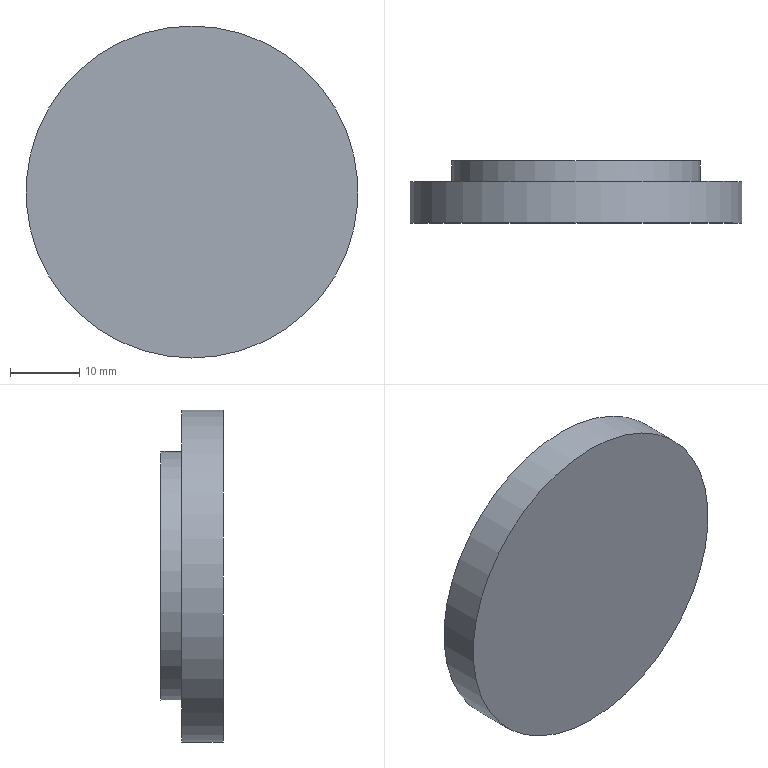Part | STEP file | zhoutaoφ36 | 1 solid | 7 faces | box 48 x 9 x 48 mm | volume 11498 mm3 | plane 4 | cylinder 3 | commonest cylinder face diameters 32 x1 36 x1 48 x1
STEP:
#1=CARTESIAN_POINT('',(0.,0.,0.));
#2=DIRECTION('',(0.,0.,1.));
#3=DIRECTION('',(1.,0.,0.));
#4=AXIS2_PLACEMENT_3D('',#1,#2,#3);
#5=CARTESIAN_POINT('',(0.,6.,24.));
#6=VERTEX_POINT('',#5);
#7=CARTESIAN_POINT('',(0.,6.,0.));
#8=DIRECTION('',(0.,1.,0.));
#9=DIRECTION('',(0.,0.,1.));
#10=AXIS2_PLACEMENT_3D('',#7,#8,#9);
#11=CIRCLE('',#10,24.);
#12=CARTESIAN_POINT('',(0.,6.,0.));
#13=DIRECTION('',(0.,-1.,0.));
#14=DIRECTION('',(0.,0.,-1.));
#15=AXIS2_PLACEMENT_3D('',#12,#13,#14);
#16=CYLINDRICAL_SURFACE('',#15,24.);
#17=CARTESIAN_POINT('',(9.425,0.));
#18=DIRECTION('',(-1.,0.));
#19=VECTOR('',#18,1.);
#20=LINE('',#17,#19);
#21=(GEOMETRIC_REPRESENTATION_CONTEXT(2)PARAMETRIC_REPRESENTATION_CONTEXT()REPRESENTATION_CONTEXT('',''));
#22=DEFINITIONAL_REPRESENTATION('',(#20),#21);
#23=PCURVE('',#16,#22);
#24=CARTESIAN_POINT('',(0.,6.,0.));
#25=DIRECTION('',(0.,1.,0.));
#26=DIRECTION('',(0.,0.,1.));
#27=AXIS2_PLACEMENT_3D('',#24,#25,#26);
#28=PLANE('',#27);
#29=CARTESIAN_POINT('',(0.,0.));
#30=DIRECTION('',(1.,0.));
#31=AXIS2_PLACEMENT_2D('',#29,#30);
#32=CIRCLE('',#31,24.);
#33=(GEOMETRIC_REPRESENTATION_CONTEXT(2)PARAMETRIC_REPRESENTATION_CONTEXT()REPRESENTATION_CONTEXT('',''));
#34=DEFINITIONAL_REPRESENTATION('',(#32),#33);
#35=PCURVE('',#28,#34);
#36=SURFACE_CURVE('',#11,(#23,#35),.PCURVE_S1.);
#37=EDGE_CURVE('',#6,#6,#36,.T.);
#38=ORIENTED_EDGE('',*,*,#37,.F.);
#39=CARTESIAN_POINT('',(0.,0.,24.));
#40=VERTEX_POINT('',#39);
#41=CARTESIAN_POINT('',(0.,6.,24.));
#42=CARTESIAN_POINT('',(0.,0.,24.));
#43=B_SPLINE_CURVE_WITH_KNOTS('',1,(#41,#42),.UNSPECIFIED.,.F.,.F.,(2,2),(0.,6.),.PIECEWISE_BEZIER_KNOTS.);
#44=CARTESIAN_POINT('',(9.425,0.));
#45=DIRECTION('',(0.,1.));
#46=VECTOR('',#45,1.);
#47=LINE('',#44,#46);
#48=(GEOMETRIC_REPRESENTATION_CONTEXT(2)PARAMETRIC_REPRESENTATION_CONTEXT()REPRESENTATION_CONTEXT('',''));
#49=DEFINITIONAL_REPRESENTATION('',(#47),#48);
#50=PCURVE('',#16,#49);
#51=CARTESIAN_POINT('',(3.142,0.));
#52=DIRECTION('',(0.,1.));
#53=VECTOR('',#52,1.);
#54=LINE('',#51,#53);
#55=(GEOMETRIC_REPRESENTATION_CONTEXT(2)PARAMETRIC_REPRESENTATION_CONTEXT()REPRESENTATION_CONTEXT('',''));
#56=DEFINITIONAL_REPRESENTATION('',(#54),#55);
#57=PCURVE('',#16,#56);
#58=SEAM_CURVE('',#43,(#50,#57),.PCURVE_S1.);
#59=EDGE_CURVE('',#6,#40,#58,.T.);
#60=ORIENTED_EDGE('',*,*,#59,.T.);
#61=CARTESIAN_POINT('',(0.,0.,0.));
#62=DIRECTION('',(0.,1.,0.));
#63=DIRECTION('',(0.,0.,1.));
#64=AXIS2_PLACEMENT_3D('',#61,#62,#63);
#65=CIRCLE('',#64,24.);
#66=CARTESIAN_POINT('',(9.425,6.));
#67=DIRECTION('',(-1.,0.));
#68=VECTOR('',#67,1.);
#69=LINE('',#66,#68);
#70=(GEOMETRIC_REPRESENTATION_CONTEXT(2)PARAMETRIC_REPRESENTATION_CONTEXT()REPRESENTATION_CONTEXT('',''));
#71=DEFINITIONAL_REPRESENTATION('',(#69),#70);
#72=PCURVE('',#16,#71);
#73=CARTESIAN_POINT('',(0.,0.,0.));
#74=DIRECTION('',(0.,1.,0.));
#75=DIRECTION('',(0.,0.,1.));
#76=AXIS2_PLACEMENT_3D('',#73,#74,#75);
#77=PLANE('',#76);
#78=CARTESIAN_POINT('',(0.,0.));
#79=DIRECTION('',(1.,0.));
#80=AXIS2_PLACEMENT_2D('',#78,#79);
#81=CIRCLE('',#80,24.);
#82=(GEOMETRIC_REPRESENTATION_CONTEXT(2)PARAMETRIC_REPRESENTATION_CONTEXT()REPRESENTATION_CONTEXT('',''));
#83=DEFINITIONAL_REPRESENTATION('',(#81),#82);
#84=PCURVE('',#77,#83);
#85=SURFACE_CURVE('',#65,(#72,#84),.PCURVE_S1.);
#86=EDGE_CURVE('',#40,#40,#85,.T.);
#87=ORIENTED_EDGE('',*,*,#86,.T.);
#88=ORIENTED_EDGE('',*,*,#59,.F.);
#89=EDGE_LOOP('',(#38,#60,#87,#88));
#90=FACE_BOUND('',#89,.T.);
#91=ADVANCED_FACE('',(#90),#16,.T.);
#92=CARTESIAN_POINT('',(0.,6.,18.));
#93=VERTEX_POINT('',#92);
#94=CARTESIAN_POINT('',(0.,6.,0.));
#95=DIRECTION('',(0.,1.,0.));
#96=DIRECTION('',(0.,0.,1.));
#97=AXIS2_PLACEMENT_3D('',#94,#95,#96);
#98=CIRCLE('',#97,18.);
#99=CARTESIAN_POINT('',(0.,0.));
#100=DIRECTION('',(1.,0.));
#101=AXIS2_PLACEMENT_2D('',#99,#100);
#102=CIRCLE('',#101,18.);
#103=(GEOMETRIC_REPRESENTATION_CONTEXT(2)PARAMETRIC_REPRESENTATION_CONTEXT()REPRESENTATION_CONTEXT('',''));
#104=DEFINITIONAL_REPRESENTATION('',(#102),#103);
#105=PCURVE('',#28,#104);
#106=CARTESIAN_POINT('',(0.,9.,0.));
#107=DIRECTION('',(0.,-1.,0.));
#108=DIRECTION('',(0.,0.,-1.));
#109=AXIS2_PLACEMENT_3D('',#106,#107,#108);
#110=CYLINDRICAL_SURFACE('',#109,18.);
#111=CARTESIAN_POINT('',(9.425,3.));
#112=DIRECTION('',(-1.,0.));
#113=VECTOR('',#112,1.);
#114=LINE('',#111,#113);
#115=(GEOMETRIC_REPRESENTATION_CONTEXT(2)PARAMETRIC_REPRESENTATION_CONTEXT()REPRESENTATION_CONTEXT('',''));
#116=DEFINITIONAL_REPRESENTATION('',(#114),#115);
#117=PCURVE('',#110,#116);
#118=SURFACE_CURVE('',#98,(#105,#117),.PCURVE_S1.);
#119=EDGE_CURVE('',#93,#93,#118,.T.);
#120=ORIENTED_EDGE('',*,*,#119,.F.);
#121=EDGE_LOOP('',(#120));
#122=FACE_BOUND('',#121,.T.);
#123=ORIENTED_EDGE('',*,*,#37,.T.);
#124=EDGE_LOOP('',(#123));
#125=FACE_BOUND('',#124,.T.);
#126=ADVANCED_FACE('',(#122,#125),#28,.T.);
#127=ORIENTED_EDGE('',*,*,#86,.F.);
#128=EDGE_LOOP('',(#127));
#129=FACE_BOUND('',#128,.T.);
#130=ADVANCED_FACE('',(#129),#77,.F.);
#131=CARTESIAN_POINT('',(0.,9.,18.));
#132=VERTEX_POINT('',#131);
#133=CARTESIAN_POINT('',(0.,9.,0.));
#134=DIRECTION('',(0.,1.,0.));
#135=DIRECTION('',(0.,0.,1.));
#136=AXIS2_PLACEMENT_3D('',#133,#134,#135);
#137=CIRCLE('',#136,18.);
#138=CARTESIAN_POINT('',(0.,9.,0.));
#139=DIRECTION('',(0.,1.,0.));
#140=DIRECTION('',(0.,0.,1.));
#141=AXIS2_PLACEMENT_3D('',#138,#139,#140);
#142=PLANE('',#141);
#143=CARTESIAN_POINT('',(0.,0.));
#144=DIRECTION('',(1.,0.));
#145=AXIS2_PLACEMENT_2D('',#143,#144);
#146=CIRCLE('',#145,18.);
#147=(GEOMETRIC_REPRESENTATION_CONTEXT(2)PARAMETRIC_REPRESENTATION_CONTEXT()REPRESENTATION_CONTEXT('',''));
#148=DEFINITIONAL_REPRESENTATION('',(#146),#147);
#149=PCURVE('',#142,#148);
#150=CARTESIAN_POINT('',(9.425,0.));
#151=DIRECTION('',(-1.,0.));
#152=VECTOR('',#151,1.);
#153=LINE('',#150,#152);
#154=(GEOMETRIC_REPRESENTATION_CONTEXT(2)PARAMETRIC_REPRESENTATION_CONTEXT()REPRESENTATION_CONTEXT('',''));
#155=DEFINITIONAL_REPRESENTATION('',(#153),#154);
#156=PCURVE('',#110,#155);
#157=SURFACE_CURVE('',#137,(#149,#156),.PCURVE_S1.);
#158=EDGE_CURVE('',#132,#132,#157,.T.);
#159=ORIENTED_EDGE('',*,*,#158,.T.);
#160=EDGE_LOOP('',(#159));
#161=FACE_BOUND('',#160,.T.);
#162=CARTESIAN_POINT('',(0.,9.,16.));
#163=VERTEX_POINT('',#162);
#164=CARTESIAN_POINT('',(0.,9.,0.));
#165=DIRECTION('',(0.,1.,0.));
#166=DIRECTION('',(0.,0.,1.));
#167=AXIS2_PLACEMENT_3D('',#164,#165,#166);
#168=CIRCLE('',#167,16.);
#169=CARTESIAN_POINT('',(0.,0.));
#170=DIRECTION('',(1.,0.));
#171=AXIS2_PLACEMENT_2D('',#169,#170);
#172=CIRCLE('',#171,16.);
#173=(GEOMETRIC_REPRESENTATION_CONTEXT(2)PARAMETRIC_REPRESENTATION_CONTEXT()REPRESENTATION_CONTEXT('',''));
#174=DEFINITIONAL_REPRESENTATION('',(#172),#173);
#175=PCURVE('',#142,#174);
#176=CARTESIAN_POINT('',(0.,9.,0.));
#177=DIRECTION('',(0.,-1.,0.));
#178=DIRECTION('',(0.,0.,-1.));
#179=AXIS2_PLACEMENT_3D('',#176,#177,#178);
#180=CYLINDRICAL_SURFACE('',#179,16.);
#181=CARTESIAN_POINT('',(9.425,0.));
#182=DIRECTION('',(-1.,0.));
#183=VECTOR('',#182,1.);
#184=LINE('',#181,#183);
#185=(GEOMETRIC_REPRESENTATION_CONTEXT(2)PARAMETRIC_REPRESENTATION_CONTEXT()REPRESENTATION_CONTEXT('',''));
#186=DEFINITIONAL_REPRESENTATION('',(#184),#185);
#187=PCURVE('',#180,#186);
#188=SURFACE_CURVE('',#168,(#175,#187),.PCURVE_S1.);
#189=EDGE_CURVE('',#163,#163,#188,.T.);
#190=ORIENTED_EDGE('',*,*,#189,.F.);
#191=EDGE_LOOP('',(#190));
#192=FACE_BOUND('',#191,.T.);
#193=ADVANCED_FACE('',(#161,#192),#142,.T.);
#194=ORIENTED_EDGE('',*,*,#158,.F.);
#195=CARTESIAN_POINT('',(0.,9.,18.));
#196=CARTESIAN_POINT('',(0.,6.,18.));
#197=B_SPLINE_CURVE_WITH_KNOTS('',1,(#195,#196),.UNSPECIFIED.,.F.,.F.,(2,2),(0.,3.),.PIECEWISE_BEZIER_KNOTS.);
#198=CARTESIAN_POINT('',(9.425,0.));
#199=DIRECTION('',(0.,1.));
#200=VECTOR('',#199,1.);
#201=LINE('',#198,#200);
#202=(GEOMETRIC_REPRESENTATION_CONTEXT(2)PARAMETRIC_REPRESENTATION_CONTEXT()REPRESENTATION_CONTEXT('',''));
#203=DEFINITIONAL_REPRESENTATION('',(#201),#202);
#204=PCURVE('',#110,#203);
#205=CARTESIAN_POINT('',(3.142,0.));
#206=DIRECTION('',(0.,1.));
#207=VECTOR('',#206,1.);
#208=LINE('',#205,#207);
#209=(GEOMETRIC_REPRESENTATION_CONTEXT(2)PARAMETRIC_REPRESENTATION_CONTEXT()REPRESENTATION_CONTEXT('',''));
#210=DEFINITIONAL_REPRESENTATION('',(#208),#209);
#211=PCURVE('',#110,#210);
#212=SEAM_CURVE('',#197,(#204,#211),.PCURVE_S1.);
#213=EDGE_CURVE('',#132,#93,#212,.T.);
#214=ORIENTED_EDGE('',*,*,#213,.T.);
#215=ORIENTED_EDGE('',*,*,#119,.T.);
#216=ORIENTED_EDGE('',*,*,#213,.F.);
#217=EDGE_LOOP('',(#194,#214,#215,#216));
#218=FACE_BOUND('',#217,.T.);
#219=ADVANCED_FACE('',(#218),#110,.T.);
#220=ORIENTED_EDGE('',*,*,#189,.F.);
#221=CARTESIAN_POINT('',(0.,6.,16.));
#222=VERTEX_POINT('',#221);
#223=CARTESIAN_POINT('',(0.,9.,16.));
#224=CARTESIAN_POINT('',(0.,6.,16.));
#225=B_SPLINE_CURVE_WITH_KNOTS('',1,(#223,#224),.UNSPECIFIED.,.F.,.F.,(2,2),(0.,3.),.PIECEWISE_BEZIER_KNOTS.);
#226=CARTESIAN_POINT('',(9.425,0.));
#227=DIRECTION('',(0.,1.));
#228=VECTOR('',#227,1.);
#229=LINE('',#226,#228);
#230=(GEOMETRIC_REPRESENTATION_CONTEXT(2)PARAMETRIC_REPRESENTATION_CONTEXT()REPRESENTATION_CONTEXT('',''));
#231=DEFINITIONAL_REPRESENTATION('',(#229),#230);
#232=PCURVE('',#180,#231);
#233=CARTESIAN_POINT('',(3.142,0.));
#234=DIRECTION('',(0.,1.));
#235=VECTOR('',#234,1.);
#236=LINE('',#233,#235);
#237=(GEOMETRIC_REPRESENTATION_CONTEXT(2)PARAMETRIC_REPRESENTATION_CONTEXT()REPRESENTATION_CONTEXT('',''));
#238=DEFINITIONAL_REPRESENTATION('',(#236),#237);
#239=PCURVE('',#180,#238);
#240=SEAM_CURVE('',#225,(#232,#239),.PCURVE_S1.);
#241=EDGE_CURVE('',#163,#222,#240,.T.);
#242=ORIENTED_EDGE('',*,*,#241,.T.);
#243=CARTESIAN_POINT('',(0.,6.,0.));
#244=DIRECTION('',(0.,-1.,0.));
#245=DIRECTION('',(0.,0.,1.));
#246=AXIS2_PLACEMENT_3D('',#243,#244,#245);
#247=CIRCLE('',#246,16.);
#248=CARTESIAN_POINT('',(3.142,3.));
#249=DIRECTION('',(1.,0.));
#250=VECTOR('',#249,1.);
#251=LINE('',#248,#250);
#252=(GEOMETRIC_REPRESENTATION_CONTEXT(2)PARAMETRIC_REPRESENTATION_CONTEXT()REPRESENTATION_CONTEXT('',''));
#253=DEFINITIONAL_REPRESENTATION('',(#251),#252);
#254=PCURVE('',#180,#253);
#255=CARTESIAN_POINT('',(0.,6.,0.));
#256=DIRECTION('',(0.,1.,0.));
#257=DIRECTION('',(0.,0.,1.));
#258=AXIS2_PLACEMENT_3D('',#255,#256,#257);
#259=PLANE('',#258);
#260=CARTESIAN_POINT('',(16.,0.));
#261=CARTESIAN_POINT('',(16.,-27.713));
#262=CARTESIAN_POINT('',(-8.,-13.856));
#263=CARTESIAN_POINT('',(-32.,0.));
#264=CARTESIAN_POINT('',(-8.,13.856));
#265=CARTESIAN_POINT('',(16.,27.713));
#266=CARTESIAN_POINT('',(16.,0.));
#267=(BOUNDED_CURVE()B_SPLINE_CURVE(2,(#260,#261,#262,#263,#264,#265,#266),.UNSPECIFIED.,.T.,.F.)B_SPLINE_CURVE_WITH_KNOTS((1,2,2,2,2,1),(-2.094,0.,2.094,4.189,6.283,8.378),.UNSPECIFIED.)CURVE()GEOMETRIC_REPRESENTATION_ITEM()RATIONAL_B_SPLINE_CURVE((1.,0.5,1.,0.5,1.,0.5,1.))REPRESENTATION_ITEM(''));
#268=(GEOMETRIC_REPRESENTATION_CONTEXT(2)PARAMETRIC_REPRESENTATION_CONTEXT()REPRESENTATION_CONTEXT('',''));
#269=DEFINITIONAL_REPRESENTATION('',(#267),#268);
#270=PCURVE('',#259,#269);
#271=SURFACE_CURVE('',#247,(#254,#270),.PCURVE_S1.);
#272=EDGE_CURVE('',#222,#222,#271,.T.);
#273=ORIENTED_EDGE('',*,*,#272,.F.);
#274=ORIENTED_EDGE('',*,*,#241,.F.);
#275=EDGE_LOOP('',(#220,#242,#273,#274));
#276=FACE_BOUND('',#275,.F.);
#277=ADVANCED_FACE('',(#276),#180,.F.);
#278=ORIENTED_EDGE('',*,*,#272,.F.);
#279=EDGE_LOOP('',(#278));
#280=FACE_BOUND('',#279,.T.);
#281=ADVANCED_FACE('',(#280),#259,.T.);
#282=CLOSED_SHELL('',(#91,#126,#130,#193,#219,#277,#281));
#283=MANIFOLD_SOLID_BREP('',#282);
#284=(LENGTH_UNIT()NAMED_UNIT(*)SI_UNIT(.MILLI.,.METRE.));
#285=UNCERTAINTY_MEASURE_WITH_UNIT(LENGTH_MEASURE(0.00001),#284,'','');
#286=(NAMED_UNIT(*)PLANE_ANGLE_UNIT()SI_UNIT($,.RADIAN.));
#287=(NAMED_UNIT(*)SI_UNIT($,.STERADIAN.)SOLID_ANGLE_UNIT());
#288=(GEOMETRIC_REPRESENTATION_CONTEXT(3)GLOBAL_UNCERTAINTY_ASSIGNED_CONTEXT((#285))GLOBAL_UNIT_ASSIGNED_CONTEXT((#284,#286,#287))REPRESENTATION_CONTEXT('',''));
#289=ADVANCED_BREP_SHAPE_REPRESENTATION('',(#4,#283),#288);